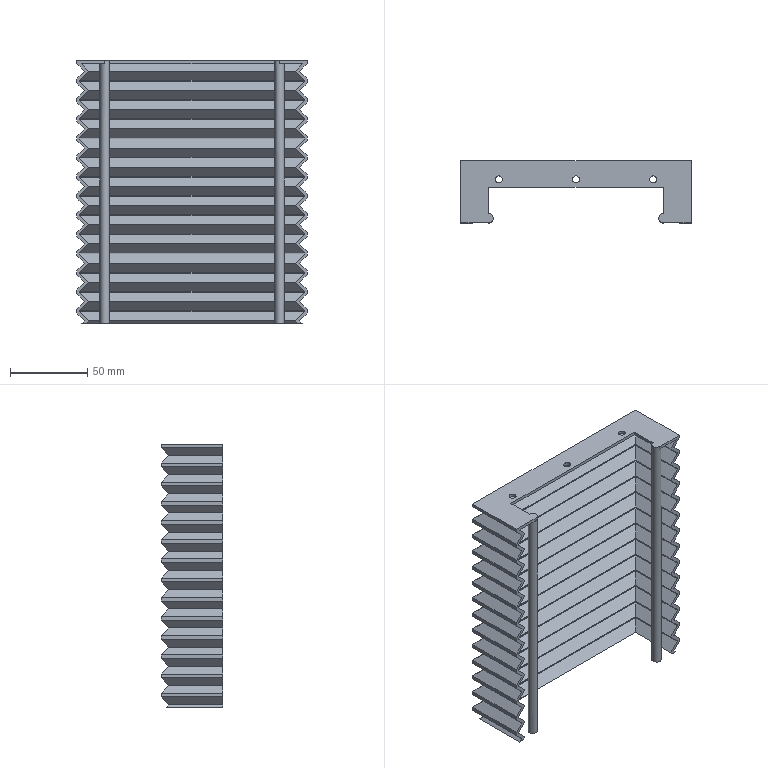Part | SolidWorks | features BaseBody 1, ICE 1 | 1 solid | 269 faces | box 149 x 40 x 170 mm | volume 114701 mm3 | plane 259 | cylinder 10 | commonest cylinder face diameters 4.5 x6 6 x4